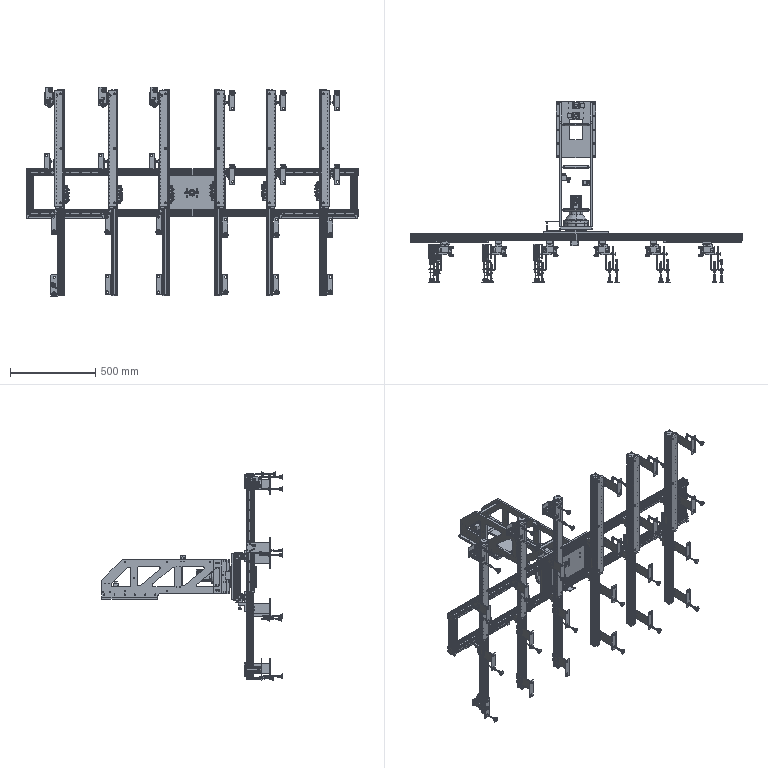Part | SolidWorks | features ReferencePattern 4, CompositeCurve 1, DerivedHolePattern 1 | 319 solids | 29035 faces | volume 20673869 mm3 | plane 11962 | cylinder 8996 | cone 4964 | spline 3075 | torus 38 | commonest cylinder face diameters 4.1 x486 4 x481 10 x388 6 x380 8 x368 7 x363